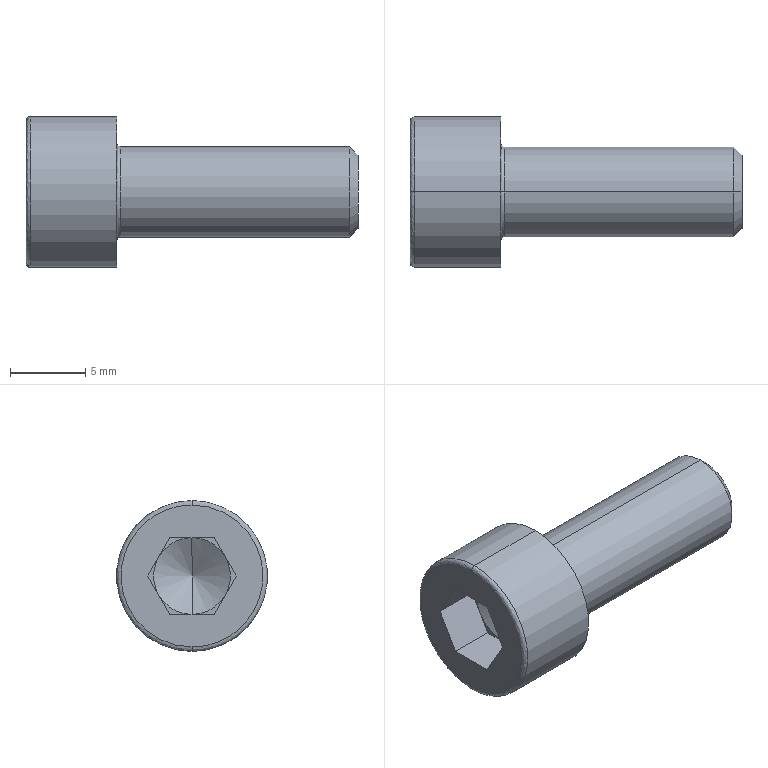Part | STEP file | 0229_306_M6x16 | 1 solid | 27 faces | box 22 x 10 x 10 mm | volume 843.509 mm3 | plane 15 | spline 4 | cylinder 4 | cone 4 | commonest cylinder face diameters 6 x2 10 x2